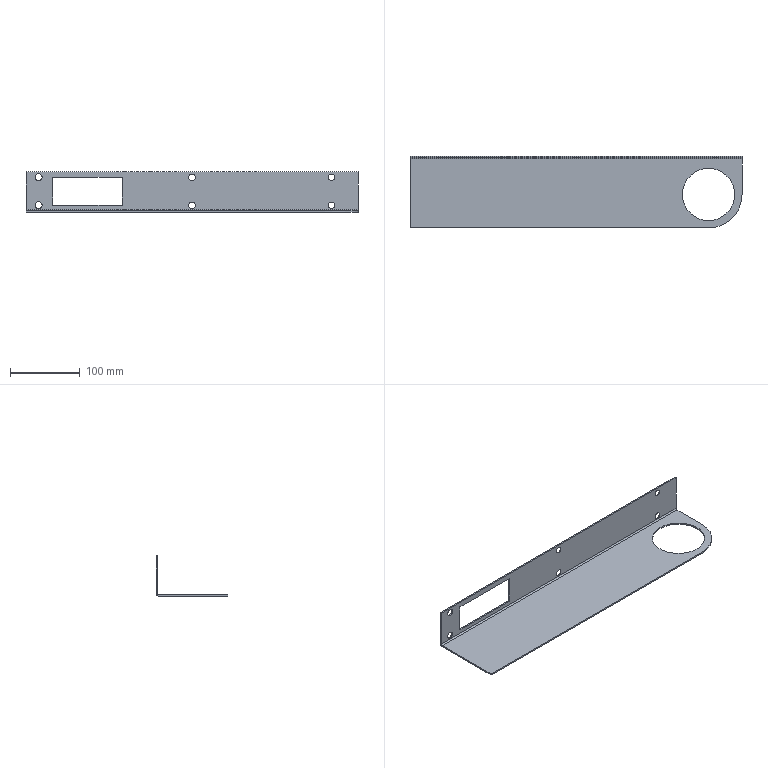Part | NX | features solid 2 | 1 solid | 29 faces | box 476 x 103 x 58 mm | volume 131195 mm3 | plane 12 | cylinder 9 | cone 8 | commonest cylinder face diameters 10 x4 75.2 x2 4 x1 8 x1 96 x1
STEP:
#1=CARTESIAN_POINT('',(-860.,-1582.,980.));
#2=VERTEX_POINT('',#1);
#3=CARTESIAN_POINT('',(-860.,-1580.,980.));
#4=VERTEX_POINT('',#3);
#5=CARTESIAN_POINT('',(-860.,-2070.458,980.));
#6=DIRECTION('',(0.,1.,0.));
#7=VECTOR('',#6,1000.);
#8=LINE('',#5,#7);
#9=EDGE_CURVE('',#2,#4,#8,.T.);
#10=ORIENTED_EDGE('',*,*,#9,.F.);
#11=CARTESIAN_POINT('',(-860.,-1582.,970.));
#12=VERTEX_POINT('',#11);
#13=CARTESIAN_POINT('',(-860.,-1582.,975.));
#14=DIRECTION('',(0.,1.,0.));
#15=DIRECTION('',(0.,0.,-1.));
#16=AXIS2_PLACEMENT_3D('',#13,#14,#15);
#17=CIRCLE('',#16,5.);
#18=EDGE_CURVE('',#12,#2,#17,.T.);
#19=ORIENTED_EDGE('',*,*,#18,.F.);
#20=CARTESIAN_POINT('',(-860.,-1580.,970.));
#21=VERTEX_POINT('',#20);
#22=CARTESIAN_POINT('',(-860.,-2070.458,970.));
#23=DIRECTION('',(0.,1.,0.));
#24=VECTOR('',#23,1000.);
#25=LINE('',#22,#24);
#26=EDGE_CURVE('',#21,#12,#25,.F.);
#27=ORIENTED_EDGE('',*,*,#26,.F.);
#28=CARTESIAN_POINT('',(-860.,-1580.,975.));
#29=DIRECTION('',(0.,1.,0.));
#30=DIRECTION('',(-1.,0.,0.));
#31=AXIS2_PLACEMENT_3D('',#28,#29,#30);
#32=CIRCLE('',#31,5.);
#33=EDGE_CURVE('',#21,#4,#32,.T.);
#34=ORIENTED_EDGE('',*,*,#33,.T.);
#35=EDGE_LOOP('',(#10,#19,#27,#34));
#36=FACE_BOUND('',#35,.T.);
#37=CARTESIAN_POINT('',(-860.,-2070.458,975.));
#38=DIRECTION('',(0.,1.,0.));
#39=DIRECTION('',(0.,0.,-1.));
#40=AXIS2_PLACEMENT_3D('',#37,#38,#39);
#41=CYLINDRICAL_SURFACE('',#40,5.);
#42=ADVANCED_FACE('',(#36),#41,.F.);
#43=CARTESIAN_POINT('',(-860.,-1582.,1020.));
#44=VERTEX_POINT('',#43);
#45=CARTESIAN_POINT('',(-860.,-1580.,1020.));
#46=VERTEX_POINT('',#45);
#47=CARTESIAN_POINT('',(-860.,-2070.458,1020.));
#48=DIRECTION('',(0.,1.,0.));
#49=VECTOR('',#48,1000.);
#50=LINE('',#47,#49);
#51=EDGE_CURVE('',#44,#46,#50,.T.);
#52=ORIENTED_EDGE('',*,*,#51,.F.);
#53=CARTESIAN_POINT('',(-860.,-1582.,1010.));
#54=VERTEX_POINT('',#53);
#55=CARTESIAN_POINT('',(-860.,-1582.,1015.));
#56=DIRECTION('',(0.,1.,0.));
#57=DIRECTION('',(0.,0.,-1.));
#58=AXIS2_PLACEMENT_3D('',#55,#56,#57);
#59=CIRCLE('',#58,5.);
#60=EDGE_CURVE('',#54,#44,#59,.T.);
#61=ORIENTED_EDGE('',*,*,#60,.F.);
#62=CARTESIAN_POINT('',(-860.,-1580.,1010.));
#63=VERTEX_POINT('',#62);
#64=CARTESIAN_POINT('',(-860.,-2070.458,1010.));
#65=DIRECTION('',(0.,1.,0.));
#66=VECTOR('',#65,1000.);
#67=LINE('',#64,#66);
#68=EDGE_CURVE('',#63,#54,#67,.F.);
#69=ORIENTED_EDGE('',*,*,#68,.F.);
#70=CARTESIAN_POINT('',(-860.,-1580.,1015.));
#71=DIRECTION('',(0.,1.,0.));
#72=DIRECTION('',(-1.,0.,0.));
#73=AXIS2_PLACEMENT_3D('',#70,#71,#72);
#74=CIRCLE('',#73,5.);
#75=EDGE_CURVE('',#63,#46,#74,.T.);
#76=ORIENTED_EDGE('',*,*,#75,.T.);
#77=EDGE_LOOP('',(#52,#61,#69,#76));
#78=FACE_BOUND('',#77,.T.);
#79=CARTESIAN_POINT('',(-860.,-2070.458,1015.));
#80=DIRECTION('',(0.,1.,0.));
#81=DIRECTION('',(0.,0.,-1.));
#82=AXIS2_PLACEMENT_3D('',#79,#80,#81);
#83=CYLINDRICAL_SURFACE('',#82,5.);
#84=ADVANCED_FACE('',(#78),#83,.F.);
#85=CARTESIAN_POINT('',(-440.,-1582.,1010.389));
#86=VERTEX_POINT('',#85);
#87=CARTESIAN_POINT('',(-440.,-1580.,1008.65));
#88=VERTEX_POINT('',#87);
#89=CARTESIAN_POINT('',(-440.,-1580.,1008.65));
#90=DIRECTION('',(0.,0.7547,-0.6561));
#91=VECTOR('',#90,1000.);
#92=LINE('',#89,#91);
#93=EDGE_CURVE('',#86,#88,#92,.T.);
#94=ORIENTED_EDGE('',*,*,#93,.F.);
#95=CARTESIAN_POINT('',(-440.,-1582.,1019.611));
#96=VERTEX_POINT('',#95);
#97=CARTESIAN_POINT('',(-440.,-1582.,1015.));
#98=DIRECTION('',(0.,-1.,0.));
#99=DIRECTION('',(0.,0.,-1.));
#100=AXIS2_PLACEMENT_3D('',#97,#98,#99);
#101=CIRCLE('',#100,4.611);
#102=EDGE_CURVE('',#86,#96,#101,.T.);
#103=ORIENTED_EDGE('',*,*,#102,.T.);
#104=CARTESIAN_POINT('',(-440.,-1580.,1021.35));
#105=VERTEX_POINT('',#104);
#106=CARTESIAN_POINT('',(-440.,-1580.,1021.35));
#107=DIRECTION('',(0.,0.7547,0.6561));
#108=VECTOR('',#107,1000.);
#109=LINE('',#106,#108);
#110=EDGE_CURVE('',#105,#96,#109,.F.);
#111=ORIENTED_EDGE('',*,*,#110,.F.);
#112=CARTESIAN_POINT('',(-440.,-1580.,1015.));
#113=DIRECTION('',(0.,1.,0.));
#114=DIRECTION('',(0.,0.,1.));
#115=AXIS2_PLACEMENT_3D('',#112,#113,#114);
#116=CIRCLE('',#115,6.35);
#117=EDGE_CURVE('',#105,#88,#116,.T.);
#118=ORIENTED_EDGE('',*,*,#117,.T.);
#119=EDGE_LOOP('',(#94,#103,#111,#118));
#120=FACE_BOUND('',#119,.T.);
#121=CARTESIAN_POINT('',(-440.,-1580.,1015.));
#122=DIRECTION('',(0.,1.,0.));
#123=DIRECTION('',(0.,0.,1.));
#124=AXIS2_PLACEMENT_3D('',#121,#122,#123);
#125=CONICAL_SURFACE('',#124,6.35,0.7156);
#126=ADVANCED_FACE('',(#120),#125,.F.);
#127=CARTESIAN_POINT('',(-640.,-1580.014,968.662));
#128=VERTEX_POINT('',#127);
#129=CARTESIAN_POINT('',(-640.,-1582.,970.389));
#130=VERTEX_POINT('',#129);
#131=CARTESIAN_POINT('',(-640.,-1580.,968.65));
#132=DIRECTION('',(0.,0.7547,-0.6561));
#133=VECTOR('',#132,1000.);
#134=LINE('',#131,#133);
#135=EDGE_CURVE('',#128,#130,#134,.F.);
#136=ORIENTED_EDGE('',*,*,#135,.T.);
#137=CARTESIAN_POINT('',(-640.,-1582.,979.611));
#138=VERTEX_POINT('',#137);
#139=CARTESIAN_POINT('',(-640.,-1582.,975.));
#140=DIRECTION('',(0.,-1.,0.));
#141=DIRECTION('',(0.,0.,-1.));
#142=AXIS2_PLACEMENT_3D('',#139,#140,#141);
#143=CIRCLE('',#142,4.611);
#144=EDGE_CURVE('',#130,#138,#143,.T.);
#145=ORIENTED_EDGE('',*,*,#144,.T.);
#146=CARTESIAN_POINT('',(-640.,-1580.,981.35));
#147=VERTEX_POINT('',#146);
#148=CARTESIAN_POINT('',(-640.,-1580.,981.35));
#149=DIRECTION('',(0.,0.7547,0.6561));
#150=VECTOR('',#149,1000.);
#151=LINE('',#148,#150);
#152=EDGE_CURVE('',#138,#147,#151,.T.);
#153=ORIENTED_EDGE('',*,*,#152,.T.);
#154=CARTESIAN_POINT('',(-637.921,-1580.,969.));
#155=VERTEX_POINT('',#154);
#156=CARTESIAN_POINT('',(-640.,-1580.,975.));
#157=DIRECTION('',(0.,1.,0.));
#158=DIRECTION('',(0.,0.,1.));
#159=AXIS2_PLACEMENT_3D('',#156,#157,#158);
#160=CIRCLE('',#159,6.35);
#161=EDGE_CURVE('',#147,#155,#160,.T.);
#162=ORIENTED_EDGE('',*,*,#161,.T.);
#163=CARTESIAN_POINT('',(-640.,-1580.014,968.662));
#164=CARTESIAN_POINT('',(-639.265,-1580.014,968.662));
#165=CARTESIAN_POINT('',(-638.572,-1580.,968.775));
#166=CARTESIAN_POINT('',(-637.921,-1580.,969.));
#167=B_SPLINE_CURVE_WITH_KNOTS('',3,(#163,#164,#165,#166),.UNSPECIFIED.,.F.,.F.,(4,4),(0.,1.),.UNSPECIFIED.);
#168=EDGE_CURVE('',#128,#155,#167,.T.);
#169=ORIENTED_EDGE('',*,*,#168,.F.);
#170=EDGE_LOOP('',(#136,#145,#153,#162,#169));
#171=FACE_BOUND('',#170,.T.);
#172=CARTESIAN_POINT('',(-640.,-1580.,975.));
#173=DIRECTION('',(0.,1.,0.));
#174=DIRECTION('',(0.,0.,1.));
#175=AXIS2_PLACEMENT_3D('',#172,#173,#174);
#176=CONICAL_SURFACE('',#175,6.35,0.7156);
#177=ADVANCED_FACE('',(#171),#176,.F.);
#178=CARTESIAN_POINT('',(-640.,-1582.,1010.389));
#179=VERTEX_POINT('',#178);
#180=CARTESIAN_POINT('',(-640.,-1580.,1008.65));
#181=VERTEX_POINT('',#180);
#182=CARTESIAN_POINT('',(-640.,-1580.,1008.65));
#183=DIRECTION('',(0.,0.7547,-0.6561));
#184=VECTOR('',#183,1000.);
#185=LINE('',#182,#184);
#186=EDGE_CURVE('',#179,#181,#185,.T.);
#187=ORIENTED_EDGE('',*,*,#186,.F.);
#188=CARTESIAN_POINT('',(-640.,-1582.,1019.611));
#189=VERTEX_POINT('',#188);
#190=CARTESIAN_POINT('',(-640.,-1582.,1015.));
#191=DIRECTION('',(0.,-1.,0.));
#192=DIRECTION('',(0.,0.,-1.));
#193=AXIS2_PLACEMENT_3D('',#190,#191,#192);
#194=CIRCLE('',#193,4.611);
#195=EDGE_CURVE('',#179,#189,#194,.T.);
#196=ORIENTED_EDGE('',*,*,#195,.T.);
#197=CARTESIAN_POINT('',(-640.,-1580.,1021.35));
#198=VERTEX_POINT('',#197);
#199=CARTESIAN_POINT('',(-640.,-1580.,1021.35));
#200=DIRECTION('',(0.,0.7547,0.6561));
#201=VECTOR('',#200,1000.);
#202=LINE('',#199,#201);
#203=EDGE_CURVE('',#198,#189,#202,.F.);
#204=ORIENTED_EDGE('',*,*,#203,.F.);
#205=CARTESIAN_POINT('',(-640.,-1580.,1015.));
#206=DIRECTION('',(0.,1.,0.));
#207=DIRECTION('',(0.,0.,1.));
#208=AXIS2_PLACEMENT_3D('',#205,#206,#207);
#209=CIRCLE('',#208,6.35);
#210=EDGE_CURVE('',#198,#181,#209,.T.);
#211=ORIENTED_EDGE('',*,*,#210,.T.);
#212=EDGE_LOOP('',(#187,#196,#204,#211));
#213=FACE_BOUND('',#212,.T.);
#214=CARTESIAN_POINT('',(-640.,-1580.,1015.));
#215=DIRECTION('',(0.,1.,0.));
#216=DIRECTION('',(0.,0.,1.));
#217=AXIS2_PLACEMENT_3D('',#214,#215,#216);
#218=CONICAL_SURFACE('',#217,6.35,0.7156);
#219=ADVANCED_FACE('',(#213),#218,.F.);
#220=CARTESIAN_POINT('',(-440.,-1582.,970.389));
#221=VERTEX_POINT('',#220);
#222=CARTESIAN_POINT('',(-440.,-1580.014,968.662));
#223=VERTEX_POINT('',#222);
#224=CARTESIAN_POINT('',(-440.,-1580.,968.65));
#225=DIRECTION('',(0.,0.7547,-0.6561));
#226=VECTOR('',#225,1000.);
#227=LINE('',#224,#226);
#228=EDGE_CURVE('',#221,#223,#227,.T.);
#229=ORIENTED_EDGE('',*,*,#228,.F.);
#230=CARTESIAN_POINT('',(-440.,-1582.,979.611));
#231=VERTEX_POINT('',#230);
#232=CARTESIAN_POINT('',(-440.,-1582.,975.));
#233=DIRECTION('',(0.,-1.,0.));
#234=DIRECTION('',(0.,0.,-1.));
#235=AXIS2_PLACEMENT_3D('',#232,#233,#234);
#236=CIRCLE('',#235,4.611);
#237=EDGE_CURVE('',#221,#231,#236,.T.);
#238=ORIENTED_EDGE('',*,*,#237,.T.);
#239=CARTESIAN_POINT('',(-440.,-1580.,981.35));
#240=VERTEX_POINT('',#239);
#241=CARTESIAN_POINT('',(-440.,-1580.,981.35));
#242=DIRECTION('',(0.,0.7547,0.6561));
#243=VECTOR('',#242,1000.);
#244=LINE('',#241,#243);
#245=EDGE_CURVE('',#240,#231,#244,.F.);
#246=ORIENTED_EDGE('',*,*,#245,.F.);
#247=CARTESIAN_POINT('',(-437.921,-1580.,969.));
#248=VERTEX_POINT('',#247);
#249=CARTESIAN_POINT('',(-440.,-1580.,975.));
#250=DIRECTION('',(0.,1.,0.));
#251=DIRECTION('',(0.,0.,1.));
#252=AXIS2_PLACEMENT_3D('',#249,#250,#251);
#253=CIRCLE('',#252,6.35);
#254=EDGE_CURVE('',#240,#248,#253,.T.);
#255=ORIENTED_EDGE('',*,*,#254,.T.);
#256=CARTESIAN_POINT('',(-440.,-1580.014,968.662));
#257=CARTESIAN_POINT('',(-439.265,-1580.014,968.662));
#258=CARTESIAN_POINT('',(-438.572,-1580.,968.775));
#259=CARTESIAN_POINT('',(-437.921,-1580.,969.));
#260=B_SPLINE_CURVE_WITH_KNOTS('',3,(#256,#257,#258,#259),.UNSPECIFIED.,.F.,.F.,(4,4),(0.,1.),.UNSPECIFIED.);
#261=EDGE_CURVE('',#223,#248,#260,.T.);
#262=ORIENTED_EDGE('',*,*,#261,.F.);
#263=EDGE_LOOP('',(#229,#238,#246,#255,#262));
#264=FACE_BOUND('',#263,.T.);
#265=CARTESIAN_POINT('',(-440.,-1580.,975.));
#266=DIRECTION('',(0.,1.,0.));
#267=DIRECTION('',(0.,0.,1.));
#268=AXIS2_PLACEMENT_3D('',#265,#266,#267);
#269=CONICAL_SURFACE('',#268,6.35,0.7156);
#270=ADVANCED_FACE('',(#264),#269,.F.);
#271=CARTESIAN_POINT('',(-740.,-1582.,1015.));
#272=VERTEX_POINT('',#271);
#273=CARTESIAN_POINT('',(-740.,-1580.,1015.));
#274=VERTEX_POINT('',#273);
#275=CARTESIAN_POINT('',(-740.,-1983.694,1015.));
#276=DIRECTION('',(0.,1.,0.));
#277=VECTOR('',#276,1000.);
#278=LINE('',#275,#277);
#279=EDGE_CURVE('',#272,#274,#278,.T.);
#280=ORIENTED_EDGE('',*,*,#279,.F.);
#281=CARTESIAN_POINT('',(-840.,-1582.,1015.));
#282=VERTEX_POINT('',#281);
#283=CARTESIAN_POINT('',(-472.,-1582.,1015.));
#284=DIRECTION('',(-1.,0.,0.));
#285=VECTOR('',#284,1000.);
#286=LINE('',#283,#285);
#287=EDGE_CURVE('',#272,#282,#286,.T.);
#288=ORIENTED_EDGE('',*,*,#287,.T.);
#289=CARTESIAN_POINT('',(-840.,-1580.,1015.));
#290=VERTEX_POINT('',#289);
#291=CARTESIAN_POINT('',(-840.,-1983.694,1015.));
#292=DIRECTION('',(0.,1.,0.));
#293=VECTOR('',#292,1000.);
#294=LINE('',#291,#293);
#295=EDGE_CURVE('',#282,#290,#294,.T.);
#296=ORIENTED_EDGE('',*,*,#295,.T.);
#297=CARTESIAN_POINT('',(-740.,-1580.,1015.));
#298=DIRECTION('',(-1.,0.,0.));
#299=VECTOR('',#298,1000.);
#300=LINE('',#297,#299);
#301=EDGE_CURVE('',#274,#290,#300,.T.);
#302=ORIENTED_EDGE('',*,*,#301,.F.);
#303=EDGE_LOOP('',(#280,#288,#296,#302));
#304=FACE_BOUND('',#303,.T.);
#305=CARTESIAN_POINT('',(-740.,-1983.694,1015.));
#306=DIRECTION('',(0.,0.,1.));
#307=DIRECTION('',(0.,-1.,0.));
#308=AXIS2_PLACEMENT_3D('',#305,#306,#307);
#309=PLANE('',#308);
#310=ADVANCED_FACE('',(#304),#309,.F.);
#311=CARTESIAN_POINT('',(-740.,-1582.,975.));
#312=VERTEX_POINT('',#311);
#313=CARTESIAN_POINT('',(-740.,-1580.,975.));
#314=VERTEX_POINT('',#313);
#315=CARTESIAN_POINT('',(-740.,-1983.694,975.));
#316=DIRECTION('',(0.,1.,0.));
#317=VECTOR('',#316,1000.);
#318=LINE('',#315,#317);
#319=EDGE_CURVE('',#312,#314,#318,.T.);
#320=ORIENTED_EDGE('',*,*,#319,.F.);
#321=CARTESIAN_POINT('',(-740.,-1582.,965.));
#322=DIRECTION('',(0.,0.,1.));
#323=VECTOR('',#322,1000.);
#324=LINE('',#321,#323);
#325=EDGE_CURVE('',#312,#272,#324,.T.);
#326=ORIENTED_EDGE('',*,*,#325,.T.);
#327=ORIENTED_EDGE('',*,*,#279,.T.);
#328=CARTESIAN_POINT('',(-740.,-1580.,975.));
#329=DIRECTION('',(0.,0.,1.));
#330=VECTOR('',#329,1000.);
#331=LINE('',#328,#330);
#332=EDGE_CURVE('',#314,#274,#331,.T.);
#333=ORIENTED_EDGE('',*,*,#332,.F.);
#334=EDGE_LOOP('',(#320,#326,#327,#333));
#335=FACE_BOUND('',#334,.T.);
#336=CARTESIAN_POINT('',(-740.,-1983.694,975.));
#337=DIRECTION('',(1.,0.,0.));
#338=DIRECTION('',(0.,1.,0.));
#339=AXIS2_PLACEMENT_3D('',#336,#337,#338);
#340=PLANE('',#339);
#341=ADVANCED_FACE('',(#335),#340,.F.);
#342=CARTESIAN_POINT('',(-840.,-1582.,975.));
#343=VERTEX_POINT('',#342);
#344=CARTESIAN_POINT('',(-840.,-1580.,975.));
#345=VERTEX_POINT('',#344);
#346=CARTESIAN_POINT('',(-840.,-1983.694,975.));
#347=DIRECTION('',(0.,1.,0.));
#348=VECTOR('',#347,1000.);
#349=LINE('',#346,#348);
#350=EDGE_CURVE('',#343,#345,#349,.T.);
#351=ORIENTED_EDGE('',*,*,#350,.F.);
#352=CARTESIAN_POINT('',(-472.,-1582.,975.));
#353=DIRECTION('',(1.,0.,0.));
#354=VECTOR('',#353,1000.);
#355=LINE('',#352,#354);
#356=EDGE_CURVE('',#343,#312,#355,.T.);
#357=ORIENTED_EDGE('',*,*,#356,.T.);
#358=ORIENTED_EDGE('',*,*,#319,.T.);
#359=CARTESIAN_POINT('',(-840.,-1580.,975.));
#360=DIRECTION('',(1.,0.,0.));
#361=VECTOR('',#360,1000.);
#362=LINE('',#359,#361);
#363=EDGE_CURVE('',#345,#314,#362,.T.);
#364=ORIENTED_EDGE('',*,*,#363,.F.);
#365=EDGE_LOOP('',(#351,#357,#358,#364));
#366=FACE_BOUND('',#365,.T.);
#367=CARTESIAN_POINT('',(-840.,-1983.694,975.));
#368=DIRECTION('',(0.,0.,-1.));
#369=DIRECTION('',(0.,-1.,0.));
#370=AXIS2_PLACEMENT_3D('',#367,#368,#369);
#371=PLANE('',#370);
#372=ADVANCED_FACE('',(#366),#371,.F.);
#373=ORIENTED_EDGE('',*,*,#295,.F.);
#374=CARTESIAN_POINT('',(-840.,-1582.,965.));
#375=DIRECTION('',(0.,0.,-1.));
#376=VECTOR('',#375,1000.);
#377=LINE('',#374,#376);
#378=EDGE_CURVE('',#282,#343,#377,.T.);
#379=ORIENTED_EDGE('',*,*,#378,.T.);
#380=ORIENTED_EDGE('',*,*,#350,.T.);
#381=CARTESIAN_POINT('',(-840.,-1580.,1015.));
#382=DIRECTION('',(0.,0.,-1.));
#383=VECTOR('',#382,1000.);
#384=LINE('',#381,#383);
#385=EDGE_CURVE('',#290,#345,#384,.T.);
#386=ORIENTED_EDGE('',*,*,#385,.F.);
#387=EDGE_LOOP('',(#373,#379,#380,#386));
#388=FACE_BOUND('',#387,.T.);
#389=CARTESIAN_POINT('',(-840.,-1983.694,1015.));
#390=DIRECTION('',(-1.,0.,0.));
#391=DIRECTION('',(0.,1.,0.));
#392=AXIS2_PLACEMENT_3D('',#389,#390,#391);
#393=PLANE('',#392);
#394=ADVANCED_FACE('',(#388),#393,.F.);
#395=CARTESIAN_POINT('',(-450.,-1672.6,967.));
#396=VERTEX_POINT('',#395);
#397=CARTESIAN_POINT('',(-450.,-1672.6,965.));
#398=VERTEX_POINT('',#397);
#399=CARTESIAN_POINT('',(-450.,-1672.6,563.306));
#400=DIRECTION('',(0.,0.,1.));
#401=VECTOR('',#400,1000.);
#402=LINE('',#399,#401);
#403=EDGE_CURVE('',#396,#398,#402,.F.);
#404=ORIENTED_EDGE('',*,*,#403,.T.);
#405=CARTESIAN_POINT('',(-450.,-1597.4,965.));
#406=VERTEX_POINT('',#405);
#407=CARTESIAN_POINT('',(-450.,-1635.,965.));
#408=DIRECTION('',(0.,0.,1.));
#409=DIRECTION('',(0.,-1.,0.));
#410=AXIS2_PLACEMENT_3D('',#407,#408,#409);
#411=CIRCLE('',#410,37.6);
#412=EDGE_CURVE('',#406,#398,#411,.T.);
#413=ORIENTED_EDGE('',*,*,#412,.F.);
#414=CARTESIAN_POINT('',(-450.,-1597.4,967.));
#415=VERTEX_POINT('',#414);
#416=CARTESIAN_POINT('',(-450.,-1597.4,563.306));
#417=DIRECTION('',(0.,0.,1.));
#418=VECTOR('',#417,1000.);
#419=LINE('',#416,#418);
#420=EDGE_CURVE('',#406,#415,#419,.T.);
#421=ORIENTED_EDGE('',*,*,#420,.T.);
#422=CARTESIAN_POINT('',(-450.,-1635.,967.));
#423=DIRECTION('',(0.,0.,-1.));
#424=DIRECTION('',(0.,1.,0.));
#425=AXIS2_PLACEMENT_3D('',#422,#423,#424);
#426=CIRCLE('',#425,37.6);
#427=EDGE_CURVE('',#396,#415,#426,.T.);
#428=ORIENTED_EDGE('',*,*,#427,.F.);
#429=EDGE_LOOP('',(#404,#413,#421,#428));
#430=FACE_BOUND('',#429,.T.);
#431=CARTESIAN_POINT('',(-450.,-1635.,563.306));
#432=DIRECTION('',(0.,0.,1.));
#433=DIRECTION('',(0.,1.,0.));
#434=AXIS2_PLACEMENT_3D('',#431,#432,#433);
#435=CYLINDRICAL_SURFACE('',#434,37.6);
#436=ADVANCED_FACE('',(#430),#435,.F.);
#437=CARTESIAN_POINT('',(-402.,-1635.,967.));
#438=VERTEX_POINT('',#437);
#439=CARTESIAN_POINT('',(-402.,-1635.,965.));
#440=VERTEX_POINT('',#439);
#441=CARTESIAN_POINT('',(-402.,-1635.,965.));
#442=DIRECTION('',(0.,0.,-1.));
#443=VECTOR('',#442,1000.);
#444=LINE('',#441,#443);
#445=EDGE_CURVE('',#438,#440,#444,.T.);
#446=ORIENTED_EDGE('',*,*,#445,.F.);
#447=CARTESIAN_POINT('',(-450.,-1683.,967.));
#448=VERTEX_POINT('',#447);
#449=CARTESIAN_POINT('',(-450.,-1635.,967.));
#450=DIRECTION('',(0.,0.,-1.));
#451=DIRECTION('',(0.,-1.,0.));
#452=AXIS2_PLACEMENT_3D('',#449,#450,#451);
#453=CIRCLE('',#452,48.);
#454=EDGE_CURVE('',#438,#448,#453,.T.);
#455=ORIENTED_EDGE('',*,*,#454,.T.);
#456=CARTESIAN_POINT('',(-450.,-1683.,965.));
#457=VERTEX_POINT('',#456);
#458=CARTESIAN_POINT('',(-450.,-1683.,965.));
#459=DIRECTION('',(0.,0.,-1.));
#460=VECTOR('',#459,1000.);
#461=LINE('',#458,#460);
#462=EDGE_CURVE('',#448,#457,#461,.T.);
#463=ORIENTED_EDGE('',*,*,#462,.T.);
#464=CARTESIAN_POINT('',(-450.,-1635.,965.));
#465=DIRECTION('',(0.,0.,-1.));
#466=DIRECTION('',(0.,-1.,0.));
#467=AXIS2_PLACEMENT_3D('',#464,#465,#466);
#468=CIRCLE('',#467,48.);
#469=EDGE_CURVE('',#440,#457,#468,.T.);
#470=ORIENTED_EDGE('',*,*,#469,.F.);
#471=EDGE_LOOP('',(#446,#455,#463,#470));
#472=FACE_BOUND('',#471,.T.);
#473=CARTESIAN_POINT('',(-450.,-1635.,965.));
#474=DIRECTION('',(0.,0.,-1.));
#475=DIRECTION('',(0.,-1.,0.));
#476=AXIS2_PLACEMENT_3D('',#473,#474,#475);
#477=CYLINDRICAL_SURFACE('',#476,48.);
#478=ADVANCED_FACE('',(#472),#477,.T.);
#479=ORIENTED_EDGE('',*,*,#287,.F.);
#480=ORIENTED_EDGE('',*,*,#325,.F.);
#481=ORIENTED_EDGE('',*,*,#356,.F.);
#482=ORIENTED_EDGE('',*,*,#378,.F.);
#483=EDGE_LOOP('',(#479,#480,#481,#482));
#484=FACE_BOUND('',#483,.T.);
#485=CARTESIAN_POINT('',(-440.,-1582.,975.));
#486=DIRECTION('',(0.,-1.,0.));
#487=DIRECTION('',(0.,0.,-1.));
#488=AXIS2_PLACEMENT_3D('',#485,#486,#487);
#489=CIRCLE('',#488,4.611);
#490=EDGE_CURVE('',#231,#221,#489,.T.);
#491=ORIENTED_EDGE('',*,*,#490,.F.);
#492=ORIENTED_EDGE('',*,*,#237,.F.);
#493=EDGE_LOOP('',(#491,#492));
#494=FACE_BOUND('',#493,.T.);
#495=CARTESIAN_POINT('',(-640.,-1582.,1015.));
#496=DIRECTION('',(0.,-1.,0.));
#497=DIRECTION('',(0.,0.,-1.));
#498=AXIS2_PLACEMENT_3D('',#495,#496,#497);
#499=CIRCLE('',#498,4.611);
#500=EDGE_CURVE('',#189,#179,#499,.T.);
#501=ORIENTED_EDGE('',*,*,#500,.F.);
#502=ORIENTED_EDGE('',*,*,#195,.F.);
#503=EDGE_LOOP('',(#501,#502));
#504=FACE_BOUND('',#503,.T.);
#505=CARTESIAN_POINT('',(-640.,-1582.,975.));
#506=DIRECTION('',(0.,-1.,0.));
#507=DIRECTION('',(0.,0.,-1.));
#508=AXIS2_PLACEMENT_3D('',#505,#506,#507);
#509=CIRCLE('',#508,4.611);
#510=EDGE_CURVE('',#138,#130,#509,.T.);
#511=ORIENTED_EDGE('',*,*,#510,.F.);
#512=ORIENTED_EDGE('',*,*,#144,.F.);
#513=EDGE_LOOP('',(#511,#512));
#514=FACE_BOUND('',#513,.T.);
#515=CARTESIAN_POINT('',(-440.,-1582.,1015.));
#516=DIRECTION('',(0.,-1.,0.));
#517=DIRECTION('',(0.,0.,-1.));
#518=AXIS2_PLACEMENT_3D('',#515,#516,#517);
#519=CIRCLE('',#518,4.611);
#520=EDGE_CURVE('',#96,#86,#519,.T.);
#521=ORIENTED_EDGE('',*,*,#520,.F.);
#522=ORIENTED_EDGE('',*,*,#102,.F.);
#523=EDGE_LOOP('',(#521,#522));
#524=FACE_BOUND('',#523,.T.);
#525=ORIENTED_EDGE('',*,*,#60,.T.);
#526=CARTESIAN_POINT('',(-860.,-1582.,1015.));
#527=DIRECTION('',(0.,1.,0.));
#528=DIRECTION('',(0.,0.,-1.));
#529=AXIS2_PLACEMENT_3D('',#526,#527,#528);
#530=CIRCLE('',#529,5.);
#531=EDGE_CURVE('',#44,#54,#530,.T.);
#532=ORIENTED_EDGE('',*,*,#531,.T.);
#533=EDGE_LOOP('',(#525,#532));
#534=FACE_BOUND('',#533,.T.);
#535=ORIENTED_EDGE('',*,*,#18,.T.);
#536=CARTESIAN_POINT('',(-860.,-1582.,975.));
#537=DIRECTION('',(0.,1.,0.));
#538=DIRECTION('',(0.,0.,-1.));
#539=AXIS2_PLACEMENT_3D('',#536,#537,#538);
#540=CIRCLE('',#539,5.);
#541=EDGE_CURVE('',#2,#12,#540,.T.);
#542=ORIENTED_EDGE('',*,*,#541,.T.);
#543=EDGE_LOOP('',(#535,#542));
#544=FACE_BOUND('',#543,.T.);
#545=CARTESIAN_POINT('',(-878.,-1582.,969.));
#546=VERTEX_POINT('',#545);
#547=CARTESIAN_POINT('',(-878.,-1582.,1023.));
#548=VERTEX_POINT('',#547);
#549=CARTESIAN_POINT('',(-878.,-1582.,965.));
#550=DIRECTION('',(0.,0.,1.));
#551=VECTOR('',#550,1000.);
#552=LINE('',#549,#551);
#553=EDGE_CURVE('',#546,#548,#552,.T.);
#554=ORIENTED_EDGE('',*,*,#553,.F.);
#555=CARTESIAN_POINT('',(-402.,-1582.,969.));
#556=VERTEX_POINT('',#555);
#557=CARTESIAN_POINT('',(-402.,-1582.,969.));
#558=DIRECTION('',(-1.,0.,0.));
#559=VECTOR('',#558,1000.);
#560=LINE('',#557,#559);
#561=EDGE_CURVE('',#556,#546,#560,.T.);
#562=ORIENTED_EDGE('',*,*,#561,.F.);
#563=CARTESIAN_POINT('',(-402.,-1582.,1023.));
#564=VERTEX_POINT('',#563);
#565=CARTESIAN_POINT('',(-402.,-1582.,965.));
#566=DIRECTION('',(0.,0.,1.));
#567=VECTOR('',#566,1000.);
#568=LINE('',#565,#567);
#569=EDGE_CURVE('',#556,#564,#568,.T.);
#570=ORIENTED_EDGE('',*,*,#569,.T.);
#571=CARTESIAN_POINT('',(-402.,-1582.,1023.));
#572=DIRECTION('',(-1.,0.,0.));
#573=VECTOR('',#572,1000.);
#574=LINE('',#571,#573);
#575=EDGE_CURVE('',#564,#548,#574,.T.);
#576=ORIENTED_EDGE('',*,*,#575,.T.);
#577=EDGE_LOOP('',(#554,#562,#570,#576));
#578=FACE_BOUND('',#577,.T.);
#579=CARTESIAN_POINT('',(-402.,-1582.,965.));
#580=DIRECTION('',(0.,1.,0.));
#581=DIRECTION('',(0.,0.,-1.));
#582=AXIS2_PLACEMENT_3D('',#579,#580,#581);
#583=PLANE('',#582);
#584=ADVANCED_FACE('',(#484,#494,#504,#514,#524,#534,#544,#578),#583,.F.);
#585=CARTESIAN_POINT('',(-878.,-1584.,967.));
#586=VERTEX_POINT('',#585);
#587=CARTESIAN_POINT('',(-878.,-1584.,969.));
#588=DIRECTION('',(1.,0.,0.));
#589=DIRECTION('',(0.,0.,-1.));
#590=AXIS2_PLACEMENT_3D('',#587,#588,#589);
#591=CIRCLE('',#590,2.);
#592=EDGE_CURVE('',#586,#546,#591,.T.);
#593=ORIENTED_EDGE('',*,*,#592,.F.);
#594=CARTESIAN_POINT('',(-402.,-1584.,967.));
#595=VERTEX_POINT('',#594);
#596=CARTESIAN_POINT('',(-402.,-1584.,967.));
#597=DIRECTION('',(-1.,0.,0.));
#598=VECTOR('',#597,1000.);
#599=LINE('',#596,#598);
#600=EDGE_CURVE('',#595,#586,#599,.T.);
#601=ORIENTED_EDGE('',*,*,#600,.F.);
#602=CARTESIAN_POINT('',(-402.,-1584.,969.));
#603=DIRECTION('',(1.,0.,0.));
#604=DIRECTION('',(0.,0.,-1.));
#605=AXIS2_PLACEMENT_3D('',#602,#603,#604);
#606=CIRCLE('',#605,2.);
#607=EDGE_CURVE('',#595,#556,#606,.T.);
#608=ORIENTED_EDGE('',*,*,#607,.T.);
#609=ORIENTED_EDGE('',*,*,#561,.T.);
#610=EDGE_LOOP('',(#593,#601,#608,#609));
#611=FACE_BOUND('',#610,.T.);
#612=CARTESIAN_POINT('',(-402.,-1584.,969.));
#613=DIRECTION('',(-1.,0.,0.));
#614=DIRECTION('',(0.,0.,-1.));
#615=AXIS2_PLACEMENT_3D('',#612,#613,#614);
#616=CYLINDRICAL_SURFACE('',#615,2.);
#617=ADVANCED_FACE('',(#611),#616,.F.);
#618=CARTESIAN_POINT('',(-450.,-1635.,967.));
#619=DIRECTION('',(0.,0.,-1.));
#620=DIRECTION('',(0.,1.,0.));
#621=AXIS2_PLACEMENT_3D('',#618,#619,#620);
#622=CIRCLE('',#621,37.6);
#623=EDGE_CURVE('',#415,#396,#622,.T.);
#624=ORIENTED_EDGE('',*,*,#623,.T.);
#625=ORIENTED_EDGE('',*,*,#427,.T.);
#626=EDGE_LOOP('',(#624,#625));
#627=FACE_BOUND('',#626,.T.);
#628=CARTESIAN_POINT('',(-402.,-1683.,967.));
#629=DIRECTION('',(0.,1.,0.));
#630=VECTOR('',#629,1000.);
#631=LINE('',#628,#630);
#632=EDGE_CURVE('',#438,#595,#631,.T.);
#633=ORIENTED_EDGE('',*,*,#632,.T.);
#634=ORIENTED_EDGE('',*,*,#600,.T.);
#635=CARTESIAN_POINT('',(-878.,-1683.,967.));
#636=VERTEX_POINT('',#635);
#637=CARTESIAN_POINT('',(-878.,-1683.,967.));
#638=DIRECTION('',(0.,1.,0.));
#639=VECTOR('',#638,1000.);
#640=LINE('',#637,#639);
#641=EDGE_CURVE('',#636,#586,#640,.T.);
#642=ORIENTED_EDGE('',*,*,#641,.F.);
#643=CARTESIAN_POINT('',(-402.,-1683.,967.));
#644=DIRECTION('',(-1.,0.,0.));
#645=VECTOR('',#644,1000.);
#646=LINE('',#643,#645);
#647=EDGE_CURVE('',#448,#636,#646,.T.);
#648=ORIENTED_EDGE('',*,*,#647,.F.);
#649=ORIENTED_EDGE('',*,*,#454,.F.);
#650=EDGE_LOOP('',(#633,#634,#642,#648,#649));
#651=FACE_BOUND('',#650,.T.);
#652=CARTESIAN_POINT('',(-402.,-1683.,967.));
#653=DIRECTION('',(0.,0.,-1.));
#654=DIRECTION('',(0.,-1.,0.));
#655=AXIS2_PLACEMENT_3D('',#652,#653,#654);
#656=PLANE('',#655);
#657=ADVANCED_FACE('',(#627,#651),#656,.F.);
#658=ORIENTED_EDGE('',*,*,#385,.T.);
#659=ORIENTED_EDGE('',*,*,#363,.T.);
#660=ORIENTED_EDGE('',*,*,#332,.T.);
#661=ORIENTED_EDGE('',*,*,#301,.T.);
#662=EDGE_LOOP('',(#658,#659,#660,#661));
#663=FACE_BOUND('',#662,.T.);
#664=ORIENTED_EDGE('',*,*,#210,.F.);
#665=CARTESIAN_POINT('',(-640.,-1580.,1015.));
#666=DIRECTION('',(0.,1.,0.));
#667=DIRECTION('',(0.,0.,1.));
#668=AXIS2_PLACEMENT_3D('',#665,#666,#667);
#669=CIRCLE('',#668,6.35);
#670=EDGE_CURVE('',#181,#198,#669,.T.);
#671=ORIENTED_EDGE('',*,*,#670,.F.);
#672=EDGE_LOOP('',(#664,#671));
#673=FACE_BOUND('',#672,.T.);
#674=ORIENTED_EDGE('',*,*,#117,.F.);
#675=CARTESIAN_POINT('',(-440.,-1580.,1015.));
#676=DIRECTION('',(0.,1.,0.));
#677=DIRECTION('',(0.,0.,1.));
#678=AXIS2_PLACEMENT_3D('',#675,#676,#677);
#679=CIRCLE('',#678,6.35);
#680=EDGE_CURVE('',#88,#105,#679,.T.);
#681=ORIENTED_EDGE('',*,*,#680,.F.);
#682=EDGE_LOOP('',(#674,#681));
#683=FACE_BOUND('',#682,.T.);
#684=ORIENTED_EDGE('',*,*,#75,.F.);
#685=CARTESIAN_POINT('',(-860.,-1580.,1015.));
#686=DIRECTION('',(0.,1.,0.));
#687=DIRECTION('',(-1.,0.,0.));
#688=AXIS2_PLACEMENT_3D('',#685,#686,#687);
#689=CIRCLE('',#688,5.);
#690=EDGE_CURVE('',#46,#63,#689,.T.);
#691=ORIENTED_EDGE('',*,*,#690,.F.);
#692=EDGE_LOOP('',(#684,#691));
#693=FACE_BOUND('',#692,.T.);
#694=ORIENTED_EDGE('',*,*,#33,.F.);
#695=CARTESIAN_POINT('',(-860.,-1580.,975.));
#696=DIRECTION('',(0.,1.,0.));
#697=DIRECTION('',(-1.,0.,0.));
#698=AXIS2_PLACEMENT_3D('',#695,#696,#697);
#699=CIRCLE('',#698,5.);
#700=EDGE_CURVE('',#4,#21,#699,.T.);
#701=ORIENTED_EDGE('',*,*,#700,.F.);
#702=EDGE_LOOP('',(#694,#701));
#703=FACE_BOUND('',#702,.T.);
#704=CARTESIAN_POINT('',(-642.079,-1580.,969.));
#705=VERTEX_POINT('',#704);
#706=CARTESIAN_POINT('',(-640.,-1580.,975.));
#707=DIRECTION('',(0.,1.,0.));
#708=DIRECTION('',(0.,0.,1.));
#709=AXIS2_PLACEMENT_3D('',#706,#707,#708);
#710=CIRCLE('',#709,6.35);
#711=EDGE_CURVE('',#705,#147,#710,.T.);
#712=ORIENTED_EDGE('',*,*,#711,.F.);
#713=CARTESIAN_POINT('',(-878.,-1580.,969.));
#714=VERTEX_POINT('',#713);
#715=CARTESIAN_POINT('',(-402.,-1580.,969.));
#716=DIRECTION('',(-1.,0.,0.));
#717=VECTOR('',#716,1000.);
#718=LINE('',#715,#717);
#719=EDGE_CURVE('',#705,#714,#718,.T.);
#720=ORIENTED_EDGE('',*,*,#719,.T.);
#721=CARTESIAN_POINT('',(-878.,-1580.,1023.));
#722=VERTEX_POINT('',#721);
#723=CARTESIAN_POINT('',(-878.,-1580.,965.));
#724=DIRECTION('',(0.,0.,1.));
#725=VECTOR('',#724,1000.);
#726=LINE('',#723,#725);
#727=EDGE_CURVE('',#714,#722,#726,.T.);
#728=ORIENTED_EDGE('',*,*,#727,.T.);
#729=CARTESIAN_POINT('',(-402.,-1580.,1023.));
#730=VERTEX_POINT('',#729);
#731=CARTESIAN_POINT('',(-402.,-1580.,1023.));
#732=DIRECTION('',(-1.,0.,0.));
#733=VECTOR('',#732,1000.);
#734=LINE('',#731,#733);
#735=EDGE_CURVE('',#730,#722,#734,.T.);
#736=ORIENTED_EDGE('',*,*,#735,.F.);
#737=CARTESIAN_POINT('',(-402.,-1580.,969.));
#738=VERTEX_POINT('',#737);
#739=CARTESIAN_POINT('',(-402.,-1580.,965.));
#740=DIRECTION('',(0.,0.,1.));
#741=VECTOR('',#740,1000.);
#742=LINE('',#739,#741);
#743=EDGE_CURVE('',#738,#730,#742,.T.);
#744=ORIENTED_EDGE('',*,*,#743,.F.);
#745=CARTESIAN_POINT('',(-402.,-1580.,969.));
#746=DIRECTION('',(-1.,0.,0.));
#747=VECTOR('',#746,1000.);
#748=LINE('',#745,#747);
#749=EDGE_CURVE('',#738,#248,#748,.T.);
#750=ORIENTED_EDGE('',*,*,#749,.T.);
#751=ORIENTED_EDGE('',*,*,#254,.F.);
#752=CARTESIAN_POINT('',(-442.079,-1580.,969.));
#753=VERTEX_POINT('',#752);
#754=CARTESIAN_POINT('',(-440.,-1580.,975.));
#755=DIRECTION('',(0.,1.,0.));
#756=DIRECTION('',(0.,0.,1.));
#757=AXIS2_PLACEMENT_3D('',#754,#755,#756);
#758=CIRCLE('',#757,6.35);
#759=EDGE_CURVE('',#753,#240,#758,.T.);
#760=ORIENTED_EDGE('',*,*,#759,.F.);
#761=CARTESIAN_POINT('',(-402.,-1580.,969.));
#762=DIRECTION('',(-1.,0.,0.));
#763=VECTOR('',#762,1000.);
#764=LINE('',#761,#763);
#765=EDGE_CURVE('',#753,#155,#764,.T.);
#766=ORIENTED_EDGE('',*,*,#765,.T.);
#767=ORIENTED_EDGE('',*,*,#161,.F.);
#768=EDGE_LOOP('',(#712,#720,#728,#736,#744,#750,#751,#760,#766,#767));
#769=FACE_BOUND('',#768,.T.);
#770=CARTESIAN_POINT('',(-402.,-1580.,965.));
#771=DIRECTION('',(0.,1.,0.));
#772=DIRECTION('',(0.,0.,-1.));
#773=AXIS2_PLACEMENT_3D('',#770,#771,#772);
#774=PLANE('',#773);
#775=ADVANCED_FACE('',(#663,#673,#683,#693,#703,#769),#774,.T.);
#776=CARTESIAN_POINT('',(-642.079,-1580.,969.));
#777=CARTESIAN_POINT('',(-641.43,-1580.,968.775));
#778=CARTESIAN_POINT('',(-640.737,-1580.014,968.663));
#779=CARTESIAN_POINT('',(-640.,-1580.014,968.662));
#780=B_SPLINE_CURVE_WITH_KNOTS('',3,(#776,#777,#778,#779),.UNSPECIFIED.,.F.,.F.,(4,4),(0.,1.),.UNSPECIFIED.);
#781=EDGE_CURVE('',#705,#128,#780,.T.);
#782=ORIENTED_EDGE('',*,*,#781,.T.);
#783=ORIENTED_EDGE('',*,*,#168,.T.);
#784=ORIENTED_EDGE('',*,*,#765,.F.);
#785=CARTESIAN_POINT('',(-442.079,-1580.,969.));
#786=CARTESIAN_POINT('',(-441.43,-1580.,968.775));
#787=CARTESIAN_POINT('',(-440.737,-1580.014,968.663));
#788=CARTESIAN_POINT('',(-440.,-1580.014,968.662));
#789=B_SPLINE_CURVE_WITH_KNOTS('',3,(#785,#786,#787,#788),.UNSPECIFIED.,.F.,.F.,(4,4),(0.,1.),.UNSPECIFIED.);
#790=EDGE_CURVE('',#753,#223,#789,.T.);
#791=ORIENTED_EDGE('',*,*,#790,.T.);
#792=ORIENTED_EDGE('',*,*,#261,.T.);
#793=ORIENTED_EDGE('',*,*,#749,.F.);
#794=CARTESIAN_POINT('',(-402.,-1584.,965.));
#795=VERTEX_POINT('',#794);
#796=CARTESIAN_POINT('',(-402.,-1584.,969.));
#797=DIRECTION('',(1.,0.,0.));
#798=DIRECTION('',(0.,0.,1.));
#799=AXIS2_PLACEMENT_3D('',#796,#797,#798);
#800=CIRCLE('',#799,4.);
#801=EDGE_CURVE('',#795,#738,#800,.T.);
#802=ORIENTED_EDGE('',*,*,#801,.F.);
#803=CARTESIAN_POINT('',(-878.,-1584.,965.));
#804=VERTEX_POINT('',#803);
#805=CARTESIAN_POINT('',(-402.,-1584.,965.));
#806=DIRECTION('',(-1.,0.,0.));
#807=VECTOR('',#806,1000.);
#808=LINE('',#805,#807);
#809=EDGE_CURVE('',#795,#804,#808,.T.);
#810=ORIENTED_EDGE('',*,*,#809,.T.);
#811=CARTESIAN_POINT('',(-878.,-1584.,969.));
#812=DIRECTION('',(1.,0.,0.));
#813=DIRECTION('',(0.,0.,1.));
#814=AXIS2_PLACEMENT_3D('',#811,#812,#813);
#815=CIRCLE('',#814,4.);
#816=EDGE_CURVE('',#804,#714,#815,.T.);
#817=ORIENTED_EDGE('',*,*,#816,.T.);
#818=ORIENTED_EDGE('',*,*,#719,.F.);
#819=EDGE_LOOP('',(#782,#783,#784,#791,#792,#793,#802,#810,#817,#818));
#820=FACE_BOUND('',#819,.T.);
#821=CARTESIAN_POINT('',(-402.,-1584.,969.));
#822=DIRECTION('',(-1.,0.,0.));
#823=DIRECTION('',(0.,0.,-1.));
#824=AXIS2_PLACEMENT_3D('',#821,#822,#823);
#825=CYLINDRICAL_SURFACE('',#824,4.);
#826=ADVANCED_FACE('',(#820),#825,.T.);
#827=ORIENTED_EDGE('',*,*,#412,.T.);
#828=CARTESIAN_POINT('',(-450.,-1635.,965.));
#829=DIRECTION('',(0.,0.,1.));
#830=DIRECTION('',(0.,-1.,0.));
#831=AXIS2_PLACEMENT_3D('',#828,#829,#830);
#832=CIRCLE('',#831,37.6);
#833=EDGE_CURVE('',#398,#406,#832,.T.);
#834=ORIENTED_EDGE('',*,*,#833,.T.);
#835=EDGE_LOOP('',(#827,#834));
#836=FACE_BOUND('',#835,.T.);
#837=ORIENTED_EDGE('',*,*,#469,.T.);
#838=CARTESIAN_POINT('',(-878.,-1683.,965.));
#839=VERTEX_POINT('',#838);
#840=CARTESIAN_POINT('',(-402.,-1683.,965.));
#841=DIRECTION('',(-1.,0.,0.));
#842=VECTOR('',#841,1000.);
#843=LINE('',#840,#842);
#844=EDGE_CURVE('',#457,#839,#843,.T.);
#845=ORIENTED_EDGE('',*,*,#844,.T.);
#846=CARTESIAN_POINT('',(-878.,-1683.,965.));
#847=DIRECTION('',(0.,1.,0.));
#848=VECTOR('',#847,1000.);
#849=LINE('',#846,#848);
#850=EDGE_CURVE('',#839,#804,#849,.T.);
#851=ORIENTED_EDGE('',*,*,#850,.T.);
#852=ORIENTED_EDGE('',*,*,#809,.F.);
#853=CARTESIAN_POINT('',(-402.,-1683.,965.));
#854=DIRECTION('',(0.,1.,0.));
#855=VECTOR('',#854,1000.);
#856=LINE('',#853,#855);
#857=EDGE_CURVE('',#440,#795,#856,.T.);
#858=ORIENTED_EDGE('',*,*,#857,.F.);
#859=EDGE_LOOP('',(#837,#845,#851,#852,#858));
#860=FACE_BOUND('',#859,.T.);
#861=CARTESIAN_POINT('',(-402.,-1683.,965.));
#862=DIRECTION('',(0.,0.,-1.));
#863=DIRECTION('',(0.,-1.,0.));
#864=AXIS2_PLACEMENT_3D('',#861,#862,#863);
#865=PLANE('',#864);
#866=ADVANCED_FACE('',(#836,#860),#865,.T.);
#867=ORIENTED_EDGE('',*,*,#850,.F.);
#868=CARTESIAN_POINT('',(-878.,-1683.,965.));
#869=DIRECTION('',(0.,0.,-1.));
#870=VECTOR('',#869,1000.);
#871=LINE('',#868,#870);
#872=EDGE_CURVE('',#636,#839,#871,.T.);
#873=ORIENTED_EDGE('',*,*,#872,.F.);
#874=ORIENTED_EDGE('',*,*,#641,.T.);
#875=ORIENTED_EDGE('',*,*,#592,.T.);
#876=ORIENTED_EDGE('',*,*,#553,.T.);
#877=CARTESIAN_POINT('',(-878.,-1580.,1023.));
#878=DIRECTION('',(0.,1.,0.));
#879=VECTOR('',#878,1000.);
#880=LINE('',#877,#879);
#881=EDGE_CURVE('',#548,#722,#880,.T.);
#882=ORIENTED_EDGE('',*,*,#881,.T.);
#883=ORIENTED_EDGE('',*,*,#727,.F.);
#884=ORIENTED_EDGE('',*,*,#816,.F.);
#885=EDGE_LOOP('',(#867,#873,#874,#875,#876,#882,#883,#884));
#886=FACE_BOUND('',#885,.T.);
#887=CARTESIAN_POINT('',(-878.,-1683.,965.));
#888=DIRECTION('',(1.,0.,0.));
#889=DIRECTION('',(0.,0.,-1.));
#890=AXIS2_PLACEMENT_3D('',#887,#888,#889);
#891=PLANE('',#890);
#892=ADVANCED_FACE('',(#886),#891,.F.);
#893=CARTESIAN_POINT('',(-402.,-1580.,1023.));
#894=DIRECTION('',(0.,1.,0.));
#895=VECTOR('',#894,1000.);
#896=LINE('',#893,#895);
#897=EDGE_CURVE('',#564,#730,#896,.T.);
#898=ORIENTED_EDGE('',*,*,#897,.T.);
#899=ORIENTED_EDGE('',*,*,#735,.T.);
#900=ORIENTED_EDGE('',*,*,#881,.F.);
#901=ORIENTED_EDGE('',*,*,#575,.F.);
#902=EDGE_LOOP('',(#898,#899,#900,#901));
#903=FACE_BOUND('',#902,.T.);
#904=CARTESIAN_POINT('',(-402.,-1580.,1023.));
#905=DIRECTION('',(0.,0.,1.));
#906=DIRECTION('',(0.,-1.,0.));
#907=AXIS2_PLACEMENT_3D('',#904,#905,#906);
#908=PLANE('',#907);
#909=ADVANCED_FACE('',(#903),#908,.T.);
#910=ORIENTED_EDGE('',*,*,#647,.T.);
#911=ORIENTED_EDGE('',*,*,#872,.T.);
#912=ORIENTED_EDGE('',*,*,#844,.F.);
#913=ORIENTED_EDGE('',*,*,#462,.F.);
#914=EDGE_LOOP('',(#910,#911,#912,#913));
#915=FACE_BOUND('',#914,.T.);
#916=CARTESIAN_POINT('',(-402.,-1683.,965.));
#917=DIRECTION('',(0.,1.,0.));
#918=DIRECTION('',(0.,0.,-1.));
#919=AXIS2_PLACEMENT_3D('',#916,#917,#918);
#920=PLANE('',#919);
#921=ADVANCED_FACE('',(#915),#920,.F.);
#922=ORIENTED_EDGE('',*,*,#857,.T.);
#923=ORIENTED_EDGE('',*,*,#801,.T.);
#924=ORIENTED_EDGE('',*,*,#743,.T.);
#925=ORIENTED_EDGE('',*,*,#897,.F.);
#926=ORIENTED_EDGE('',*,*,#569,.F.);
#927=ORIENTED_EDGE('',*,*,#607,.F.);
#928=ORIENTED_EDGE('',*,*,#632,.F.);
#929=ORIENTED_EDGE('',*,*,#445,.T.);
#930=EDGE_LOOP('',(#922,#923,#924,#925,#926,#927,#928,#929));
#931=FACE_BOUND('',#930,.T.);
#932=CARTESIAN_POINT('',(-402.,-1580.,965.));
#933=DIRECTION('',(1.,0.,0.));
#934=DIRECTION('',(0.,0.,-1.));
#935=AXIS2_PLACEMENT_3D('',#932,#933,#934);
#936=PLANE('',#935);
#937=ADVANCED_FACE('',(#931),#936,.T.);
#938=ORIENTED_EDGE('',*,*,#833,.F.);
#939=ORIENTED_EDGE('',*,*,#403,.F.);
#940=ORIENTED_EDGE('',*,*,#623,.F.);
#941=ORIENTED_EDGE('',*,*,#420,.F.);
#942=EDGE_LOOP('',(#938,#939,#940,#941));
#943=FACE_BOUND('',#942,.T.);
#944=CARTESIAN_POINT('',(-450.,-1635.,563.306));
#945=DIRECTION('',(0.,0.,1.));
#946=DIRECTION('',(0.,1.,0.));
#947=AXIS2_PLACEMENT_3D('',#944,#945,#946);
#948=CYLINDRICAL_SURFACE('',#947,37.6);
#949=ADVANCED_FACE('',(#943),#948,.F.);
#950=ORIENTED_EDGE('',*,*,#490,.T.);
#951=ORIENTED_EDGE('',*,*,#228,.T.);
#952=ORIENTED_EDGE('',*,*,#790,.F.);
#953=ORIENTED_EDGE('',*,*,#759,.T.);
#954=ORIENTED_EDGE('',*,*,#245,.T.);
#955=EDGE_LOOP('',(#950,#951,#952,#953,#954));
#956=FACE_BOUND('',#955,.T.);
#957=CARTESIAN_POINT('',(-440.,-1580.,975.));
#958=DIRECTION('',(0.,1.,0.));
#959=DIRECTION('',(0.,0.,1.));
#960=AXIS2_PLACEMENT_3D('',#957,#958,#959);
#961=CONICAL_SURFACE('',#960,6.35,0.7156);
#962=ADVANCED_FACE('',(#956),#961,.F.);
#963=ORIENTED_EDGE('',*,*,#500,.T.);
#964=ORIENTED_EDGE('',*,*,#186,.T.);
#965=ORIENTED_EDGE('',*,*,#670,.T.);
#966=ORIENTED_EDGE('',*,*,#203,.T.);
#967=EDGE_LOOP('',(#963,#964,#965,#966));
#968=FACE_BOUND('',#967,.T.);
#969=CARTESIAN_POINT('',(-640.,-1580.,1015.));
#970=DIRECTION('',(0.,1.,0.));
#971=DIRECTION('',(0.,0.,1.));
#972=AXIS2_PLACEMENT_3D('',#969,#970,#971);
#973=CONICAL_SURFACE('',#972,6.35,0.7156);
#974=ADVANCED_FACE('',(#968),#973,.F.);
#975=ORIENTED_EDGE('',*,*,#510,.T.);
#976=ORIENTED_EDGE('',*,*,#135,.F.);
#977=ORIENTED_EDGE('',*,*,#781,.F.);
#978=ORIENTED_EDGE('',*,*,#711,.T.);
#979=ORIENTED_EDGE('',*,*,#152,.F.);
#980=EDGE_LOOP('',(#975,#976,#977,#978,#979));
#981=FACE_BOUND('',#980,.T.);
#982=CARTESIAN_POINT('',(-640.,-1580.,975.));
#983=DIRECTION('',(0.,1.,0.));
#984=DIRECTION('',(0.,0.,1.));
#985=AXIS2_PLACEMENT_3D('',#982,#983,#984);
#986=CONICAL_SURFACE('',#985,6.35,0.7156);
#987=ADVANCED_FACE('',(#981),#986,.F.);
#988=ORIENTED_EDGE('',*,*,#520,.T.);
#989=ORIENTED_EDGE('',*,*,#93,.T.);
#990=ORIENTED_EDGE('',*,*,#680,.T.);
#991=ORIENTED_EDGE('',*,*,#110,.T.);
#992=EDGE_LOOP('',(#988,#989,#990,#991));
#993=FACE_BOUND('',#992,.T.);
#994=CARTESIAN_POINT('',(-440.,-1580.,1015.));
#995=DIRECTION('',(0.,1.,0.));
#996=DIRECTION('',(0.,0.,1.));
#997=AXIS2_PLACEMENT_3D('',#994,#995,#996);
#998=CONICAL_SURFACE('',#997,6.35,0.7156);
#999=ADVANCED_FACE('',(#993),#998,.F.);
#1000=ORIENTED_EDGE('',*,*,#531,.F.);
#1001=ORIENTED_EDGE('',*,*,#51,.T.);
#1002=ORIENTED_EDGE('',*,*,#690,.T.);
#1003=ORIENTED_EDGE('',*,*,#68,.T.);
#1004=EDGE_LOOP('',(#1000,#1001,#1002,#1003));
#1005=FACE_BOUND('',#1004,.T.);
#1006=CARTESIAN_POINT('',(-860.,-2070.458,1015.));
#1007=DIRECTION('',(0.,1.,0.));
#1008=DIRECTION('',(0.,0.,-1.));
#1009=AXIS2_PLACEMENT_3D('',#1006,#1007,#1008);
#1010=CYLINDRICAL_SURFACE('',#1009,5.);
#1011=ADVANCED_FACE('',(#1005),#1010,.F.);
#1012=ORIENTED_EDGE('',*,*,#541,.F.);
#1013=ORIENTED_EDGE('',*,*,#9,.T.);
#1014=ORIENTED_EDGE('',*,*,#700,.T.);
#1015=ORIENTED_EDGE('',*,*,#26,.T.);
#1016=EDGE_LOOP('',(#1012,#1013,#1014,#1015));
#1017=FACE_BOUND('',#1016,.T.);
#1018=CARTESIAN_POINT('',(-860.,-2070.458,975.));
#1019=DIRECTION('',(0.,1.,0.));
#1020=DIRECTION('',(0.,0.,-1.));
#1021=AXIS2_PLACEMENT_3D('',#1018,#1019,#1020);
#1022=CYLINDRICAL_SURFACE('',#1021,5.);
#1023=ADVANCED_FACE('',(#1017),#1022,.F.);
#1024=CLOSED_SHELL('',(#42,#84,#126,#177,#219,#270,#310,#341,#372,#394,#436,#478,#584,#617,#657,#775,#826,#866,#892,#909,#921,#937,#949,#962,#974,#987,#999,#1011,#1023));
#1025=MANIFOLD_SOLID_BREP('',#1024);
#1026=(LENGTH_UNIT()NAMED_UNIT(*)SI_UNIT(.MILLI.,.METRE.));
#1027=UNCERTAINTY_MEASURE_WITH_UNIT(LENGTH_MEASURE(0.0508),#1026,'','');
#1028=(NAMED_UNIT(*)PLANE_ANGLE_UNIT()SI_UNIT($,.RADIAN.));
#1029=(NAMED_UNIT(*)SI_UNIT($,.STERADIAN.)SOLID_ANGLE_UNIT());
#1030=(GEOMETRIC_REPRESENTATION_CONTEXT(3)GLOBAL_UNCERTAINTY_ASSIGNED_CONTEXT((#1027))GLOBAL_UNIT_ASSIGNED_CONTEXT((#1026,#1028,#1029))REPRESENTATION_CONTEXT('',''));
#1031=ADVANCED_BREP_SHAPE_REPRESENTATION('',(#1025),#1030);